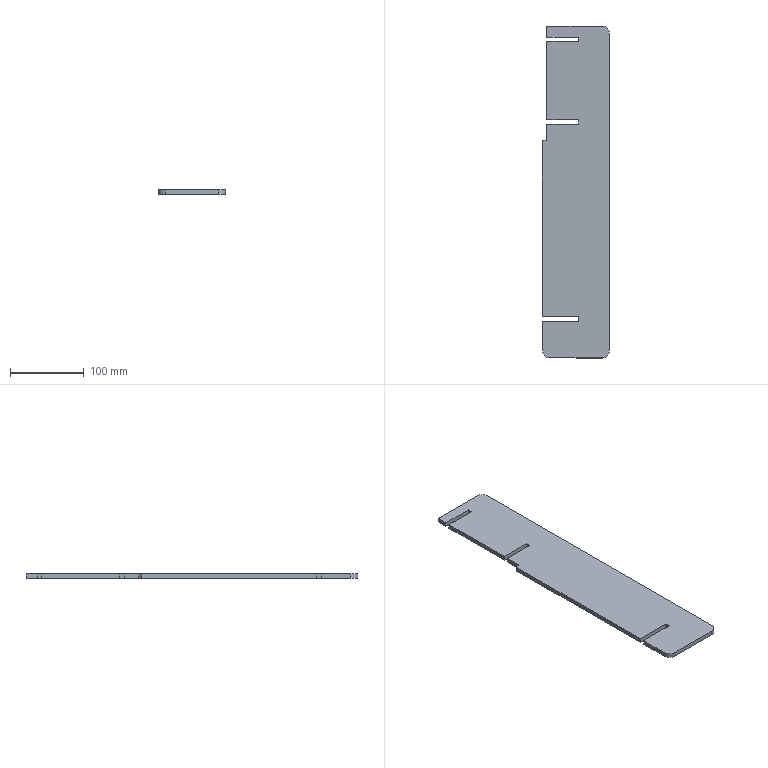Part | SolidWorks | features FlatPattern 1, SMBaseFlange 1, SheetMetal 1 | 1 solid | 25 faces | box 91 x 450 x 6 mm | volume 234874 mm3 | plane 20 | cylinder 5 | commonest cylinder face diameters 20 x3 4 x2
STEP:
#1=CARTESIAN_POINT('',(508.5,249.356,0.));
#2=VERTEX_POINT('',#1);
#3=CARTESIAN_POINT('',(508.5,234.356,0.));
#4=VERTEX_POINT('',#3);
#5=CARTESIAN_POINT('',(508.5,249.356,0.));
#6=DIRECTION('',(0.,-1.,0.));
#7=VECTOR('',#6,1000.);
#8=LINE('',#5,#7);
#9=EDGE_CURVE('',#2,#4,#8,.T.);
#10=ORIENTED_EDGE('',*,*,#9,.T.);
#11=CARTESIAN_POINT('',(508.5,234.356,6.));
#12=VERTEX_POINT('',#11);
#13=CARTESIAN_POINT('',(508.5,234.356,6.));
#14=DIRECTION('',(0.,0.,-1.));
#15=VECTOR('',#14,1000.);
#16=LINE('',#13,#15);
#17=EDGE_CURVE('',#12,#4,#16,.T.);
#18=ORIENTED_EDGE('',*,*,#17,.F.);
#19=CARTESIAN_POINT('',(508.5,249.356,6.));
#20=VERTEX_POINT('',#19);
#21=CARTESIAN_POINT('',(508.5,249.356,6.));
#22=DIRECTION('',(0.,-1.,0.));
#23=VECTOR('',#22,1000.);
#24=LINE('',#21,#23);
#25=EDGE_CURVE('',#20,#12,#24,.T.);
#26=ORIENTED_EDGE('',*,*,#25,.F.);
#27=CARTESIAN_POINT('',(508.5,249.356,6.));
#28=DIRECTION('',(0.,0.,-1.));
#29=VECTOR('',#28,1000.);
#30=LINE('',#27,#29);
#31=EDGE_CURVE('',#20,#2,#30,.T.);
#32=ORIENTED_EDGE('',*,*,#31,.T.);
#33=EDGE_LOOP('',(#10,#18,#26,#32));
#34=FACE_OUTER_BOUND('',#33,.T.);
#35=CARTESIAN_POINT('',(508.5,249.356,6.));
#36=DIRECTION('',(1.,0.,0.));
#37=DIRECTION('',(0.,0.,-1.));
#38=AXIS2_PLACEMENT_3D('',#35,#36,#37);
#39=PLANE('',#38);
#40=ADVANCED_FACE('',(#34),#39,.F.);
#41=CARTESIAN_POINT('',(551.5,234.356,0.));
#42=VERTEX_POINT('',#41);
#43=CARTESIAN_POINT('',(508.5,234.356,0.));
#44=DIRECTION('',(1.,0.,0.));
#45=VECTOR('',#44,1000.);
#46=LINE('',#43,#45);
#47=EDGE_CURVE('',#4,#42,#46,.T.);
#48=ORIENTED_EDGE('',*,*,#47,.T.);
#49=CARTESIAN_POINT('',(551.5,234.356,6.));
#50=VERTEX_POINT('',#49);
#51=CARTESIAN_POINT('',(551.5,234.356,6.));
#52=DIRECTION('',(0.,0.,-1.));
#53=VECTOR('',#52,1000.);
#54=LINE('',#51,#53);
#55=EDGE_CURVE('',#50,#42,#54,.T.);
#56=ORIENTED_EDGE('',*,*,#55,.F.);
#57=CARTESIAN_POINT('',(508.5,234.356,6.));
#58=DIRECTION('',(1.,0.,0.));
#59=VECTOR('',#58,1000.);
#60=LINE('',#57,#59);
#61=EDGE_CURVE('',#12,#50,#60,.T.);
#62=ORIENTED_EDGE('',*,*,#61,.F.);
#63=ORIENTED_EDGE('',*,*,#17,.T.);
#64=EDGE_LOOP('',(#48,#56,#62,#63));
#65=FACE_OUTER_BOUND('',#64,.T.);
#66=CARTESIAN_POINT('',(508.5,234.356,6.));
#67=DIRECTION('',(0.,1.,0.));
#68=DIRECTION('',(0.,0.,1.));
#69=AXIS2_PLACEMENT_3D('',#66,#67,#68);
#70=PLANE('',#69);
#71=ADVANCED_FACE('',(#65),#70,.F.);
#72=CARTESIAN_POINT('',(551.5,228.356,0.));
#73=VERTEX_POINT('',#72);
#74=CARTESIAN_POINT('',(551.5,234.356,0.));
#75=DIRECTION('',(0.,-1.,0.));
#76=VECTOR('',#75,1000.);
#77=LINE('',#74,#76);
#78=EDGE_CURVE('',#42,#73,#77,.T.);
#79=ORIENTED_EDGE('',*,*,#78,.T.);
#80=CARTESIAN_POINT('',(551.5,228.356,6.));
#81=VERTEX_POINT('',#80);
#82=CARTESIAN_POINT('',(551.5,228.356,6.));
#83=DIRECTION('',(0.,0.,-1.));
#84=VECTOR('',#83,1000.);
#85=LINE('',#82,#84);
#86=EDGE_CURVE('',#81,#73,#85,.T.);
#87=ORIENTED_EDGE('',*,*,#86,.F.);
#88=CARTESIAN_POINT('',(551.5,234.356,6.));
#89=DIRECTION('',(0.,-1.,0.));
#90=VECTOR('',#89,1000.);
#91=LINE('',#88,#90);
#92=EDGE_CURVE('',#50,#81,#91,.T.);
#93=ORIENTED_EDGE('',*,*,#92,.F.);
#94=ORIENTED_EDGE('',*,*,#55,.T.);
#95=EDGE_LOOP('',(#79,#87,#93,#94));
#96=FACE_OUTER_BOUND('',#95,.T.);
#97=CARTESIAN_POINT('',(551.5,234.356,6.));
#98=DIRECTION('',(1.,0.,0.));
#99=DIRECTION('',(0.,0.,-1.));
#100=AXIS2_PLACEMENT_3D('',#97,#98,#99);
#101=PLANE('',#100);
#102=ADVANCED_FACE('',(#96),#101,.F.);
#103=CARTESIAN_POINT('',(508.5,228.356,0.));
#104=VERTEX_POINT('',#103);
#105=CARTESIAN_POINT('',(551.5,228.356,0.));
#106=DIRECTION('',(-1.,0.,0.));
#107=VECTOR('',#106,1000.);
#108=LINE('',#105,#107);
#109=EDGE_CURVE('',#73,#104,#108,.T.);
#110=ORIENTED_EDGE('',*,*,#109,.T.);
#111=CARTESIAN_POINT('',(508.5,228.356,6.));
#112=VERTEX_POINT('',#111);
#113=CARTESIAN_POINT('',(508.5,228.356,6.));
#114=DIRECTION('',(0.,0.,-1.));
#115=VECTOR('',#114,1000.);
#116=LINE('',#113,#115);
#117=EDGE_CURVE('',#112,#104,#116,.T.);
#118=ORIENTED_EDGE('',*,*,#117,.F.);
#119=CARTESIAN_POINT('',(551.5,228.356,6.));
#120=DIRECTION('',(-1.,0.,0.));
#121=VECTOR('',#120,1000.);
#122=LINE('',#119,#121);
#123=EDGE_CURVE('',#81,#112,#122,.T.);
#124=ORIENTED_EDGE('',*,*,#123,.F.);
#125=ORIENTED_EDGE('',*,*,#86,.T.);
#126=EDGE_LOOP('',(#110,#118,#124,#125));
#127=FACE_OUTER_BOUND('',#126,.T.);
#128=CARTESIAN_POINT('',(551.5,228.356,6.));
#129=DIRECTION('',(0.,-1.,0.));
#130=DIRECTION('',(0.,0.,-1.));
#131=AXIS2_PLACEMENT_3D('',#128,#129,#130);
#132=PLANE('',#131);
#133=ADVANCED_FACE('',(#127),#132,.F.);
#134=CARTESIAN_POINT('',(508.5,122.356,0.));
#135=VERTEX_POINT('',#134);
#136=CARTESIAN_POINT('',(508.5,228.356,0.));
#137=DIRECTION('',(0.,-1.,0.));
#138=VECTOR('',#137,1000.);
#139=LINE('',#136,#138);
#140=EDGE_CURVE('',#104,#135,#139,.T.);
#141=ORIENTED_EDGE('',*,*,#140,.T.);
#142=CARTESIAN_POINT('',(508.5,122.356,6.));
#143=VERTEX_POINT('',#142);
#144=CARTESIAN_POINT('',(508.5,122.356,6.));
#145=DIRECTION('',(0.,0.,-1.));
#146=VECTOR('',#145,1000.);
#147=LINE('',#144,#146);
#148=EDGE_CURVE('',#143,#135,#147,.T.);
#149=ORIENTED_EDGE('',*,*,#148,.F.);
#150=CARTESIAN_POINT('',(508.5,228.356,6.));
#151=DIRECTION('',(0.,-1.,0.));
#152=VECTOR('',#151,1000.);
#153=LINE('',#150,#152);
#154=EDGE_CURVE('',#112,#143,#153,.T.);
#155=ORIENTED_EDGE('',*,*,#154,.F.);
#156=ORIENTED_EDGE('',*,*,#117,.T.);
#157=EDGE_LOOP('',(#141,#149,#155,#156));
#158=FACE_OUTER_BOUND('',#157,.T.);
#159=CARTESIAN_POINT('',(508.5,228.356,6.));
#160=DIRECTION('',(1.,0.,0.));
#161=DIRECTION('',(0.,0.,-1.));
#162=AXIS2_PLACEMENT_3D('',#159,#160,#161);
#163=PLANE('',#162);
#164=ADVANCED_FACE('',(#158),#163,.F.);
#165=CARTESIAN_POINT('',(551.5,122.356,0.));
#166=VERTEX_POINT('',#165);
#167=CARTESIAN_POINT('',(508.5,122.356,0.));
#168=DIRECTION('',(1.,0.,0.));
#169=VECTOR('',#168,1000.);
#170=LINE('',#167,#169);
#171=EDGE_CURVE('',#135,#166,#170,.T.);
#172=ORIENTED_EDGE('',*,*,#171,.T.);
#173=CARTESIAN_POINT('',(551.5,122.356,6.));
#174=VERTEX_POINT('',#173);
#175=CARTESIAN_POINT('',(551.5,122.356,6.));
#176=DIRECTION('',(0.,0.,-1.));
#177=VECTOR('',#176,1000.);
#178=LINE('',#175,#177);
#179=EDGE_CURVE('',#174,#166,#178,.T.);
#180=ORIENTED_EDGE('',*,*,#179,.F.);
#181=CARTESIAN_POINT('',(508.5,122.356,6.));
#182=DIRECTION('',(1.,0.,0.));
#183=VECTOR('',#182,1000.);
#184=LINE('',#181,#183);
#185=EDGE_CURVE('',#143,#174,#184,.T.);
#186=ORIENTED_EDGE('',*,*,#185,.F.);
#187=ORIENTED_EDGE('',*,*,#148,.T.);
#188=EDGE_LOOP('',(#172,#180,#186,#187));
#189=FACE_OUTER_BOUND('',#188,.T.);
#190=CARTESIAN_POINT('',(508.5,122.356,6.));
#191=DIRECTION('',(0.,1.,0.));
#192=DIRECTION('',(0.,0.,1.));
#193=AXIS2_PLACEMENT_3D('',#190,#191,#192);
#194=PLANE('',#193);
#195=ADVANCED_FACE('',(#189),#194,.F.);
#196=CARTESIAN_POINT('',(551.5,116.356,0.));
#197=VERTEX_POINT('',#196);
#198=CARTESIAN_POINT('',(551.5,122.356,0.));
#199=DIRECTION('',(0.,-1.,0.));
#200=VECTOR('',#199,1000.);
#201=LINE('',#198,#200);
#202=EDGE_CURVE('',#166,#197,#201,.T.);
#203=ORIENTED_EDGE('',*,*,#202,.T.);
#204=CARTESIAN_POINT('',(551.5,116.356,6.));
#205=VERTEX_POINT('',#204);
#206=CARTESIAN_POINT('',(551.5,116.356,6.));
#207=DIRECTION('',(0.,0.,-1.));
#208=VECTOR('',#207,1000.);
#209=LINE('',#206,#208);
#210=EDGE_CURVE('',#205,#197,#209,.T.);
#211=ORIENTED_EDGE('',*,*,#210,.F.);
#212=CARTESIAN_POINT('',(551.5,122.356,6.));
#213=DIRECTION('',(0.,-1.,0.));
#214=VECTOR('',#213,1000.);
#215=LINE('',#212,#214);
#216=EDGE_CURVE('',#174,#205,#215,.T.);
#217=ORIENTED_EDGE('',*,*,#216,.F.);
#218=ORIENTED_EDGE('',*,*,#179,.T.);
#219=EDGE_LOOP('',(#203,#211,#217,#218));
#220=FACE_OUTER_BOUND('',#219,.T.);
#221=CARTESIAN_POINT('',(551.5,122.356,6.));
#222=DIRECTION('',(1.,0.,0.));
#223=DIRECTION('',(0.,0.,-1.));
#224=AXIS2_PLACEMENT_3D('',#221,#222,#223);
#225=PLANE('',#224);
#226=ADVANCED_FACE('',(#220),#225,.F.);
#227=CARTESIAN_POINT('',(508.5,116.356,0.));
#228=VERTEX_POINT('',#227);
#229=CARTESIAN_POINT('',(551.5,116.356,0.));
#230=DIRECTION('',(-1.,0.,0.));
#231=VECTOR('',#230,1000.);
#232=LINE('',#229,#231);
#233=EDGE_CURVE('',#197,#228,#232,.T.);
#234=ORIENTED_EDGE('',*,*,#233,.T.);
#235=CARTESIAN_POINT('',(508.5,116.356,6.));
#236=VERTEX_POINT('',#235);
#237=CARTESIAN_POINT('',(508.5,116.356,6.));
#238=DIRECTION('',(0.,0.,-1.));
#239=VECTOR('',#238,1000.);
#240=LINE('',#237,#239);
#241=EDGE_CURVE('',#236,#228,#240,.T.);
#242=ORIENTED_EDGE('',*,*,#241,.F.);
#243=CARTESIAN_POINT('',(551.5,116.356,6.));
#244=DIRECTION('',(-1.,0.,0.));
#245=VECTOR('',#244,1000.);
#246=LINE('',#243,#245);
#247=EDGE_CURVE('',#205,#236,#246,.T.);
#248=ORIENTED_EDGE('',*,*,#247,.F.);
#249=ORIENTED_EDGE('',*,*,#210,.T.);
#250=EDGE_LOOP('',(#234,#242,#248,#249));
#251=FACE_OUTER_BOUND('',#250,.T.);
#252=CARTESIAN_POINT('',(551.5,116.356,6.));
#253=DIRECTION('',(0.,-1.,0.));
#254=DIRECTION('',(0.,0.,-1.));
#255=AXIS2_PLACEMENT_3D('',#252,#253,#254);
#256=PLANE('',#255);
#257=ADVANCED_FACE('',(#251),#256,.F.);
#258=CARTESIAN_POINT('',(508.5,96.356,0.));
#259=VERTEX_POINT('',#258);
#260=CARTESIAN_POINT('',(508.5,116.356,0.));
#261=DIRECTION('',(0.,-1.,0.));
#262=VECTOR('',#261,1000.);
#263=LINE('',#260,#262);
#264=EDGE_CURVE('',#228,#259,#263,.T.);
#265=ORIENTED_EDGE('',*,*,#264,.T.);
#266=CARTESIAN_POINT('',(508.5,96.356,6.));
#267=VERTEX_POINT('',#266);
#268=CARTESIAN_POINT('',(508.5,96.356,6.));
#269=DIRECTION('',(0.,0.,-1.));
#270=VECTOR('',#269,1000.);
#271=LINE('',#268,#270);
#272=EDGE_CURVE('',#267,#259,#271,.T.);
#273=ORIENTED_EDGE('',*,*,#272,.F.);
#274=CARTESIAN_POINT('',(508.5,116.356,6.));
#275=DIRECTION('',(0.,-1.,0.));
#276=VECTOR('',#275,1000.);
#277=LINE('',#274,#276);
#278=EDGE_CURVE('',#236,#267,#277,.T.);
#279=ORIENTED_EDGE('',*,*,#278,.F.);
#280=ORIENTED_EDGE('',*,*,#241,.T.);
#281=EDGE_LOOP('',(#265,#273,#279,#280));
#282=FACE_OUTER_BOUND('',#281,.T.);
#283=CARTESIAN_POINT('',(508.5,116.356,6.));
#284=DIRECTION('',(1.,0.,0.));
#285=DIRECTION('',(0.,0.,-1.));
#286=AXIS2_PLACEMENT_3D('',#283,#284,#285);
#287=PLANE('',#286);
#288=ADVANCED_FACE('',(#282),#287,.F.);
#289=CARTESIAN_POINT('',(506.5,94.356,0.));
#290=VERTEX_POINT('',#289);
#291=CARTESIAN_POINT('',(506.5,96.356,0.));
#292=DIRECTION('',(0.,0.,-1.));
#293=DIRECTION('',(-1.,0.,0.));
#294=AXIS2_PLACEMENT_3D('',#291,#292,#293);
#295=CIRCLE('',#294,2.);
#296=EDGE_CURVE('',#259,#290,#295,.T.);
#297=ORIENTED_EDGE('',*,*,#296,.T.);
#298=CARTESIAN_POINT('',(506.5,94.356,6.));
#299=VERTEX_POINT('',#298);
#300=CARTESIAN_POINT('',(506.5,94.356,6.));
#301=DIRECTION('',(0.,0.,-1.));
#302=VECTOR('',#301,1000.);
#303=LINE('',#300,#302);
#304=EDGE_CURVE('',#299,#290,#303,.T.);
#305=ORIENTED_EDGE('',*,*,#304,.F.);
#306=CARTESIAN_POINT('',(506.5,96.356,6.));
#307=DIRECTION('',(0.,0.,-1.));
#308=DIRECTION('',(-1.,0.,0.));
#309=AXIS2_PLACEMENT_3D('',#306,#307,#308);
#310=CIRCLE('',#309,2.);
#311=EDGE_CURVE('',#267,#299,#310,.T.);
#312=ORIENTED_EDGE('',*,*,#311,.F.);
#313=ORIENTED_EDGE('',*,*,#272,.T.);
#314=EDGE_LOOP('',(#297,#305,#312,#313));
#315=FACE_OUTER_BOUND('',#314,.T.);
#316=CARTESIAN_POINT('',(506.5,96.356,6.));
#317=DIRECTION('',(0.,0.,-1.));
#318=DIRECTION('',(-1.,0.,0.));
#319=AXIS2_PLACEMENT_3D('',#316,#317,#318);
#320=CYLINDRICAL_SURFACE('',#319,2.);
#321=ADVANCED_FACE('',(#315),#320,.F.);
#322=CARTESIAN_POINT('',(504.5,94.356,0.));
#323=VERTEX_POINT('',#322);
#324=CARTESIAN_POINT('',(506.5,94.356,0.));
#325=DIRECTION('',(-1.,0.,0.));
#326=VECTOR('',#325,1000.);
#327=LINE('',#324,#326);
#328=EDGE_CURVE('',#290,#323,#327,.T.);
#329=ORIENTED_EDGE('',*,*,#328,.T.);
#330=CARTESIAN_POINT('',(504.5,94.356,6.));
#331=VERTEX_POINT('',#330);
#332=CARTESIAN_POINT('',(504.5,94.356,6.));
#333=DIRECTION('',(0.,0.,-1.));
#334=VECTOR('',#333,1000.);
#335=LINE('',#332,#334);
#336=EDGE_CURVE('',#331,#323,#335,.T.);
#337=ORIENTED_EDGE('',*,*,#336,.F.);
#338=CARTESIAN_POINT('',(506.5,94.356,6.));
#339=DIRECTION('',(-1.,0.,0.));
#340=VECTOR('',#339,1000.);
#341=LINE('',#338,#340);
#342=EDGE_CURVE('',#299,#331,#341,.T.);
#343=ORIENTED_EDGE('',*,*,#342,.F.);
#344=ORIENTED_EDGE('',*,*,#304,.T.);
#345=EDGE_LOOP('',(#329,#337,#343,#344));
#346=FACE_OUTER_BOUND('',#345,.T.);
#347=CARTESIAN_POINT('',(506.5,94.356,6.));
#348=DIRECTION('',(0.,-1.,0.));
#349=DIRECTION('',(1.,0.,0.));
#350=AXIS2_PLACEMENT_3D('',#347,#348,#349);
#351=PLANE('',#350);
#352=ADVANCED_FACE('',(#346),#351,.F.);
#353=CARTESIAN_POINT('',(502.5,92.356,0.));
#354=VERTEX_POINT('',#353);
#355=CARTESIAN_POINT('',(504.5,92.356,0.));
#356=DIRECTION('',(0.,0.,1.));
#357=DIRECTION('',(1.,0.,0.));
#358=AXIS2_PLACEMENT_3D('',#355,#356,#357);
#359=CIRCLE('',#358,2.);
#360=EDGE_CURVE('',#323,#354,#359,.T.);
#361=ORIENTED_EDGE('',*,*,#360,.T.);
#362=CARTESIAN_POINT('',(502.5,92.356,6.));
#363=VERTEX_POINT('',#362);
#364=CARTESIAN_POINT('',(502.5,92.356,6.));
#365=DIRECTION('',(0.,0.,-1.));
#366=VECTOR('',#365,1000.);
#367=LINE('',#364,#366);
#368=EDGE_CURVE('',#363,#354,#367,.T.);
#369=ORIENTED_EDGE('',*,*,#368,.F.);
#370=CARTESIAN_POINT('',(504.5,92.356,6.));
#371=DIRECTION('',(0.,0.,1.));
#372=DIRECTION('',(1.,0.,0.));
#373=AXIS2_PLACEMENT_3D('',#370,#371,#372);
#374=CIRCLE('',#373,2.);
#375=EDGE_CURVE('',#331,#363,#374,.T.);
#376=ORIENTED_EDGE('',*,*,#375,.F.);
#377=ORIENTED_EDGE('',*,*,#336,.T.);
#378=EDGE_LOOP('',(#361,#369,#376,#377));
#379=FACE_OUTER_BOUND('',#378,.T.);
#380=CARTESIAN_POINT('',(504.5,92.356,6.));
#381=DIRECTION('',(0.,0.,-1.));
#382=DIRECTION('',(-1.,0.,0.));
#383=AXIS2_PLACEMENT_3D('',#380,#381,#382);
#384=CYLINDRICAL_SURFACE('',#383,2.);
#385=ADVANCED_FACE('',(#379),#384,.T.);
#386=CARTESIAN_POINT('',(502.5,-144.644,0.));
#387=VERTEX_POINT('',#386);
#388=CARTESIAN_POINT('',(502.5,92.356,0.));
#389=DIRECTION('',(0.,-1.,0.));
#390=VECTOR('',#389,1000.);
#391=LINE('',#388,#390);
#392=EDGE_CURVE('',#354,#387,#391,.T.);
#393=ORIENTED_EDGE('',*,*,#392,.T.);
#394=CARTESIAN_POINT('',(502.5,-144.644,6.));
#395=VERTEX_POINT('',#394);
#396=CARTESIAN_POINT('',(502.5,-144.644,6.));
#397=DIRECTION('',(0.,0.,-1.));
#398=VECTOR('',#397,1000.);
#399=LINE('',#396,#398);
#400=EDGE_CURVE('',#395,#387,#399,.T.);
#401=ORIENTED_EDGE('',*,*,#400,.F.);
#402=CARTESIAN_POINT('',(502.5,92.356,6.));
#403=DIRECTION('',(0.,-1.,0.));
#404=VECTOR('',#403,1000.);
#405=LINE('',#402,#404);
#406=EDGE_CURVE('',#363,#395,#405,.T.);
#407=ORIENTED_EDGE('',*,*,#406,.F.);
#408=ORIENTED_EDGE('',*,*,#368,.T.);
#409=EDGE_LOOP('',(#393,#401,#407,#408));
#410=FACE_OUTER_BOUND('',#409,.T.);
#411=CARTESIAN_POINT('',(502.5,92.356,6.));
#412=DIRECTION('',(1.,0.,0.));
#413=DIRECTION('',(0.,0.,-1.));
#414=AXIS2_PLACEMENT_3D('',#411,#412,#413);
#415=PLANE('',#414);
#416=ADVANCED_FACE('',(#410),#415,.F.);
#417=CARTESIAN_POINT('',(551.5,-144.644,0.));
#418=VERTEX_POINT('',#417);
#419=CARTESIAN_POINT('',(502.5,-144.644,0.));
#420=DIRECTION('',(1.,0.,0.));
#421=VECTOR('',#420,1000.);
#422=LINE('',#419,#421);
#423=EDGE_CURVE('',#387,#418,#422,.T.);
#424=ORIENTED_EDGE('',*,*,#423,.T.);
#425=CARTESIAN_POINT('',(551.5,-144.644,6.));
#426=VERTEX_POINT('',#425);
#427=CARTESIAN_POINT('',(551.5,-144.644,6.));
#428=DIRECTION('',(0.,0.,-1.));
#429=VECTOR('',#428,1000.);
#430=LINE('',#427,#429);
#431=EDGE_CURVE('',#426,#418,#430,.T.);
#432=ORIENTED_EDGE('',*,*,#431,.F.);
#433=CARTESIAN_POINT('',(502.5,-144.644,6.));
#434=DIRECTION('',(1.,0.,0.));
#435=VECTOR('',#434,1000.);
#436=LINE('',#433,#435);
#437=EDGE_CURVE('',#395,#426,#436,.T.);
#438=ORIENTED_EDGE('',*,*,#437,.F.);
#439=ORIENTED_EDGE('',*,*,#400,.T.);
#440=EDGE_LOOP('',(#424,#432,#438,#439));
#441=FACE_OUTER_BOUND('',#440,.T.);
#442=CARTESIAN_POINT('',(502.5,-144.644,6.));
#443=DIRECTION('',(0.,1.,0.));
#444=DIRECTION('',(0.,0.,1.));
#445=AXIS2_PLACEMENT_3D('',#442,#443,#444);
#446=PLANE('',#445);
#447=ADVANCED_FACE('',(#441),#446,.F.);
#448=CARTESIAN_POINT('',(551.5,-150.644,0.));
#449=VERTEX_POINT('',#448);
#450=CARTESIAN_POINT('',(551.5,-144.644,0.));
#451=DIRECTION('',(0.,-1.,0.));
#452=VECTOR('',#451,1000.);
#453=LINE('',#450,#452);
#454=EDGE_CURVE('',#418,#449,#453,.T.);
#455=ORIENTED_EDGE('',*,*,#454,.T.);
#456=CARTESIAN_POINT('',(551.5,-150.644,6.));
#457=VERTEX_POINT('',#456);
#458=CARTESIAN_POINT('',(551.5,-150.644,6.));
#459=DIRECTION('',(0.,0.,-1.));
#460=VECTOR('',#459,1000.);
#461=LINE('',#458,#460);
#462=EDGE_CURVE('',#457,#449,#461,.T.);
#463=ORIENTED_EDGE('',*,*,#462,.F.);
#464=CARTESIAN_POINT('',(551.5,-144.644,6.));
#465=DIRECTION('',(0.,-1.,0.));
#466=VECTOR('',#465,1000.);
#467=LINE('',#464,#466);
#468=EDGE_CURVE('',#426,#457,#467,.T.);
#469=ORIENTED_EDGE('',*,*,#468,.F.);
#470=ORIENTED_EDGE('',*,*,#431,.T.);
#471=EDGE_LOOP('',(#455,#463,#469,#470));
#472=FACE_OUTER_BOUND('',#471,.T.);
#473=CARTESIAN_POINT('',(551.5,-144.644,6.));
#474=DIRECTION('',(1.,0.,0.));
#475=DIRECTION('',(0.,0.,-1.));
#476=AXIS2_PLACEMENT_3D('',#473,#474,#475);
#477=PLANE('',#476);
#478=ADVANCED_FACE('',(#472),#477,.F.);
#479=CARTESIAN_POINT('',(502.5,-150.644,0.));
#480=VERTEX_POINT('',#479);
#481=CARTESIAN_POINT('',(551.5,-150.644,0.));
#482=DIRECTION('',(-1.,0.,0.));
#483=VECTOR('',#482,1000.);
#484=LINE('',#481,#483);
#485=EDGE_CURVE('',#449,#480,#484,.T.);
#486=ORIENTED_EDGE('',*,*,#485,.T.);
#487=CARTESIAN_POINT('',(502.5,-150.644,6.));
#488=VERTEX_POINT('',#487);
#489=CARTESIAN_POINT('',(502.5,-150.644,6.));
#490=DIRECTION('',(0.,0.,-1.));
#491=VECTOR('',#490,1000.);
#492=LINE('',#489,#491);
#493=EDGE_CURVE('',#488,#480,#492,.T.);
#494=ORIENTED_EDGE('',*,*,#493,.F.);
#495=CARTESIAN_POINT('',(551.5,-150.644,6.));
#496=DIRECTION('',(-1.,0.,0.));
#497=VECTOR('',#496,1000.);
#498=LINE('',#495,#497);
#499=EDGE_CURVE('',#457,#488,#498,.T.);
#500=ORIENTED_EDGE('',*,*,#499,.F.);
#501=ORIENTED_EDGE('',*,*,#462,.T.);
#502=EDGE_LOOP('',(#486,#494,#500,#501));
#503=FACE_OUTER_BOUND('',#502,.T.);
#504=CARTESIAN_POINT('',(551.5,-150.644,6.));
#505=DIRECTION('',(0.,-1.,0.));
#506=DIRECTION('',(0.,0.,-1.));
#507=AXIS2_PLACEMENT_3D('',#504,#505,#506);
#508=PLANE('',#507);
#509=ADVANCED_FACE('',(#503),#508,.F.);
#510=CARTESIAN_POINT('',(502.5,-190.644,0.));
#511=VERTEX_POINT('',#510);
#512=CARTESIAN_POINT('',(502.5,-150.644,0.));
#513=DIRECTION('',(0.,-1.,0.));
#514=VECTOR('',#513,1000.);
#515=LINE('',#512,#514);
#516=EDGE_CURVE('',#480,#511,#515,.T.);
#517=ORIENTED_EDGE('',*,*,#516,.T.);
#518=CARTESIAN_POINT('',(502.5,-190.644,6.));
#519=VERTEX_POINT('',#518);
#520=CARTESIAN_POINT('',(502.5,-190.644,6.));
#521=DIRECTION('',(0.,0.,-1.));
#522=VECTOR('',#521,1000.);
#523=LINE('',#520,#522);
#524=EDGE_CURVE('',#519,#511,#523,.T.);
#525=ORIENTED_EDGE('',*,*,#524,.F.);
#526=CARTESIAN_POINT('',(502.5,-150.644,6.));
#527=DIRECTION('',(0.,-1.,0.));
#528=VECTOR('',#527,1000.);
#529=LINE('',#526,#528);
#530=EDGE_CURVE('',#488,#519,#529,.T.);
#531=ORIENTED_EDGE('',*,*,#530,.F.);
#532=ORIENTED_EDGE('',*,*,#493,.T.);
#533=EDGE_LOOP('',(#517,#525,#531,#532));
#534=FACE_OUTER_BOUND('',#533,.T.);
#535=CARTESIAN_POINT('',(502.5,-150.644,6.));
#536=DIRECTION('',(1.,0.,0.));
#537=DIRECTION('',(0.,1.,0.));
#538=AXIS2_PLACEMENT_3D('',#535,#536,#537);
#539=PLANE('',#538);
#540=ADVANCED_FACE('',(#534),#539,.F.);
#541=CARTESIAN_POINT('',(512.5,-200.644,0.));
#542=VERTEX_POINT('',#541);
#543=CARTESIAN_POINT('',(512.5,-190.644,0.));
#544=DIRECTION('',(0.,0.,1.));
#545=DIRECTION('',(1.,0.,0.));
#546=AXIS2_PLACEMENT_3D('',#543,#544,#545);
#547=CIRCLE('',#546,10.);
#548=EDGE_CURVE('',#511,#542,#547,.T.);
#549=ORIENTED_EDGE('',*,*,#548,.T.);
#550=CARTESIAN_POINT('',(512.5,-200.644,6.));
#551=VERTEX_POINT('',#550);
#552=CARTESIAN_POINT('',(512.5,-200.644,6.));
#553=DIRECTION('',(0.,0.,-1.));
#554=VECTOR('',#553,1000.);
#555=LINE('',#552,#554);
#556=EDGE_CURVE('',#551,#542,#555,.T.);
#557=ORIENTED_EDGE('',*,*,#556,.F.);
#558=CARTESIAN_POINT('',(512.5,-190.644,6.));
#559=DIRECTION('',(0.,0.,1.));
#560=DIRECTION('',(1.,0.,0.));
#561=AXIS2_PLACEMENT_3D('',#558,#559,#560);
#562=CIRCLE('',#561,10.);
#563=EDGE_CURVE('',#519,#551,#562,.T.);
#564=ORIENTED_EDGE('',*,*,#563,.F.);
#565=ORIENTED_EDGE('',*,*,#524,.T.);
#566=EDGE_LOOP('',(#549,#557,#564,#565));
#567=FACE_OUTER_BOUND('',#566,.T.);
#568=CARTESIAN_POINT('',(512.5,-190.644,6.));
#569=DIRECTION('',(0.,0.,-1.));
#570=DIRECTION('',(-1.,0.,0.));
#571=AXIS2_PLACEMENT_3D('',#568,#569,#570);
#572=CYLINDRICAL_SURFACE('',#571,10.);
#573=ADVANCED_FACE('',(#567),#572,.T.);
#574=CARTESIAN_POINT('',(583.5,-200.644,0.));
#575=VERTEX_POINT('',#574);
#576=CARTESIAN_POINT('',(512.5,-200.644,0.));
#577=DIRECTION('',(1.,0.,0.));
#578=VECTOR('',#577,1000.);
#579=LINE('',#576,#578);
#580=EDGE_CURVE('',#542,#575,#579,.T.);
#581=ORIENTED_EDGE('',*,*,#580,.T.);
#582=CARTESIAN_POINT('',(583.5,-200.644,6.));
#583=VERTEX_POINT('',#582);
#584=CARTESIAN_POINT('',(583.5,-200.644,6.));
#585=DIRECTION('',(0.,0.,-1.));
#586=VECTOR('',#585,1000.);
#587=LINE('',#584,#586);
#588=EDGE_CURVE('',#583,#575,#587,.T.);
#589=ORIENTED_EDGE('',*,*,#588,.F.);
#590=CARTESIAN_POINT('',(512.5,-200.644,6.));
#591=DIRECTION('',(1.,0.,0.));
#592=VECTOR('',#591,1000.);
#593=LINE('',#590,#592);
#594=EDGE_CURVE('',#551,#583,#593,.T.);
#595=ORIENTED_EDGE('',*,*,#594,.F.);
#596=ORIENTED_EDGE('',*,*,#556,.T.);
#597=EDGE_LOOP('',(#581,#589,#595,#596));
#598=FACE_OUTER_BOUND('',#597,.T.);
#599=CARTESIAN_POINT('',(512.5,-200.644,6.));
#600=DIRECTION('',(0.,1.,0.));
#601=DIRECTION('',(-1.,0.,0.));
#602=AXIS2_PLACEMENT_3D('',#599,#600,#601);
#603=PLANE('',#602);
#604=ADVANCED_FACE('',(#598),#603,.F.);
#605=CARTESIAN_POINT('',(593.5,-190.644,0.));
#606=VERTEX_POINT('',#605);
#607=CARTESIAN_POINT('',(583.5,-190.644,0.));
#608=DIRECTION('',(0.,0.,1.));
#609=DIRECTION('',(1.,0.,0.));
#610=AXIS2_PLACEMENT_3D('',#607,#608,#609);
#611=CIRCLE('',#610,10.);
#612=EDGE_CURVE('',#575,#606,#611,.T.);
#613=ORIENTED_EDGE('',*,*,#612,.T.);
#614=CARTESIAN_POINT('',(593.5,-190.644,6.));
#615=VERTEX_POINT('',#614);
#616=CARTESIAN_POINT('',(593.5,-190.644,6.));
#617=DIRECTION('',(0.,0.,-1.));
#618=VECTOR('',#617,1000.);
#619=LINE('',#616,#618);
#620=EDGE_CURVE('',#615,#606,#619,.T.);
#621=ORIENTED_EDGE('',*,*,#620,.F.);
#622=CARTESIAN_POINT('',(583.5,-190.644,6.));
#623=DIRECTION('',(0.,0.,1.));
#624=DIRECTION('',(1.,0.,0.));
#625=AXIS2_PLACEMENT_3D('',#622,#623,#624);
#626=CIRCLE('',#625,10.);
#627=EDGE_CURVE('',#583,#615,#626,.T.);
#628=ORIENTED_EDGE('',*,*,#627,.F.);
#629=ORIENTED_EDGE('',*,*,#588,.T.);
#630=EDGE_LOOP('',(#613,#621,#628,#629));
#631=FACE_OUTER_BOUND('',#630,.T.);
#632=CARTESIAN_POINT('',(583.5,-190.644,6.));
#633=DIRECTION('',(0.,0.,-1.));
#634=DIRECTION('',(-1.,0.,0.));
#635=AXIS2_PLACEMENT_3D('',#632,#633,#634);
#636=CYLINDRICAL_SURFACE('',#635,10.);
#637=ADVANCED_FACE('',(#631),#636,.T.);
#638=CARTESIAN_POINT('',(593.5,239.356,0.));
#639=VERTEX_POINT('',#638);
#640=CARTESIAN_POINT('',(593.5,-190.644,0.));
#641=DIRECTION('',(0.,1.,0.));
#642=VECTOR('',#641,1000.);
#643=LINE('',#640,#642);
#644=EDGE_CURVE('',#606,#639,#643,.T.);
#645=ORIENTED_EDGE('',*,*,#644,.T.);
#646=CARTESIAN_POINT('',(593.5,239.356,6.));
#647=VERTEX_POINT('',#646);
#648=CARTESIAN_POINT('',(593.5,239.356,6.));
#649=DIRECTION('',(0.,0.,-1.));
#650=VECTOR('',#649,1000.);
#651=LINE('',#648,#650);
#652=EDGE_CURVE('',#647,#639,#651,.T.);
#653=ORIENTED_EDGE('',*,*,#652,.F.);
#654=CARTESIAN_POINT('',(593.5,-190.644,6.));
#655=DIRECTION('',(0.,1.,0.));
#656=VECTOR('',#655,1000.);
#657=LINE('',#654,#656);
#658=EDGE_CURVE('',#615,#647,#657,.T.);
#659=ORIENTED_EDGE('',*,*,#658,.F.);
#660=ORIENTED_EDGE('',*,*,#620,.T.);
#661=EDGE_LOOP('',(#645,#653,#659,#660));
#662=FACE_OUTER_BOUND('',#661,.T.);
#663=CARTESIAN_POINT('',(593.5,-190.644,6.));
#664=DIRECTION('',(-1.,0.,0.));
#665=DIRECTION('',(0.,0.,1.));
#666=AXIS2_PLACEMENT_3D('',#663,#664,#665);
#667=PLANE('',#666);
#668=ADVANCED_FACE('',(#662),#667,.F.);
#669=CARTESIAN_POINT('',(583.5,249.356,0.));
#670=VERTEX_POINT('',#669);
#671=CARTESIAN_POINT('',(583.5,239.356,0.));
#672=DIRECTION('',(0.,0.,1.));
#673=DIRECTION('',(-1.,0.,0.));
#674=AXIS2_PLACEMENT_3D('',#671,#672,#673);
#675=CIRCLE('',#674,10.);
#676=EDGE_CURVE('',#639,#670,#675,.T.);
#677=ORIENTED_EDGE('',*,*,#676,.T.);
#678=CARTESIAN_POINT('',(583.5,249.356,6.));
#679=VERTEX_POINT('',#678);
#680=CARTESIAN_POINT('',(583.5,249.356,6.));
#681=DIRECTION('',(0.,0.,-1.));
#682=VECTOR('',#681,1000.);
#683=LINE('',#680,#682);
#684=EDGE_CURVE('',#679,#670,#683,.T.);
#685=ORIENTED_EDGE('',*,*,#684,.F.);
#686=CARTESIAN_POINT('',(583.5,239.356,6.));
#687=DIRECTION('',(0.,0.,1.));
#688=DIRECTION('',(-1.,0.,0.));
#689=AXIS2_PLACEMENT_3D('',#686,#687,#688);
#690=CIRCLE('',#689,10.);
#691=EDGE_CURVE('',#647,#679,#690,.T.);
#692=ORIENTED_EDGE('',*,*,#691,.F.);
#693=ORIENTED_EDGE('',*,*,#652,.T.);
#694=EDGE_LOOP('',(#677,#685,#692,#693));
#695=FACE_OUTER_BOUND('',#694,.T.);
#696=CARTESIAN_POINT('',(583.5,239.356,6.));
#697=DIRECTION('',(0.,0.,-1.));
#698=DIRECTION('',(-1.,0.,0.));
#699=AXIS2_PLACEMENT_3D('',#696,#697,#698);
#700=CYLINDRICAL_SURFACE('',#699,10.);
#701=ADVANCED_FACE('',(#695),#700,.T.);
#702=CARTESIAN_POINT('',(583.5,249.356,0.));
#703=DIRECTION('',(-1.,0.,0.));
#704=VECTOR('',#703,1000.);
#705=LINE('',#702,#704);
#706=EDGE_CURVE('',#670,#2,#705,.T.);
#707=ORIENTED_EDGE('',*,*,#706,.T.);
#708=ORIENTED_EDGE('',*,*,#31,.F.);
#709=CARTESIAN_POINT('',(583.5,249.356,6.));
#710=DIRECTION('',(-1.,0.,0.));
#711=VECTOR('',#710,1000.);
#712=LINE('',#709,#711);
#713=EDGE_CURVE('',#679,#20,#712,.T.);
#714=ORIENTED_EDGE('',*,*,#713,.F.);
#715=ORIENTED_EDGE('',*,*,#684,.T.);
#716=EDGE_LOOP('',(#707,#708,#714,#715));
#717=FACE_OUTER_BOUND('',#716,.T.);
#718=CARTESIAN_POINT('',(583.5,249.356,6.));
#719=DIRECTION('',(0.,-1.,0.));
#720=DIRECTION('',(1.,0.,0.));
#721=AXIS2_PLACEMENT_3D('',#718,#719,#720);
#722=PLANE('',#721);
#723=ADVANCED_FACE('',(#717),#722,.F.);
#724=ORIENTED_EDGE('',*,*,#25,.T.);
#725=ORIENTED_EDGE('',*,*,#61,.T.);
#726=ORIENTED_EDGE('',*,*,#92,.T.);
#727=ORIENTED_EDGE('',*,*,#123,.T.);
#728=ORIENTED_EDGE('',*,*,#154,.T.);
#729=ORIENTED_EDGE('',*,*,#185,.T.);
#730=ORIENTED_EDGE('',*,*,#216,.T.);
#731=ORIENTED_EDGE('',*,*,#247,.T.);
#732=ORIENTED_EDGE('',*,*,#278,.T.);
#733=ORIENTED_EDGE('',*,*,#311,.T.);
#734=ORIENTED_EDGE('',*,*,#342,.T.);
#735=ORIENTED_EDGE('',*,*,#375,.T.);
#736=ORIENTED_EDGE('',*,*,#406,.T.);
#737=ORIENTED_EDGE('',*,*,#437,.T.);
#738=ORIENTED_EDGE('',*,*,#468,.T.);
#739=ORIENTED_EDGE('',*,*,#499,.T.);
#740=ORIENTED_EDGE('',*,*,#530,.T.);
#741=ORIENTED_EDGE('',*,*,#563,.T.);
#742=ORIENTED_EDGE('',*,*,#594,.T.);
#743=ORIENTED_EDGE('',*,*,#627,.T.);
#744=ORIENTED_EDGE('',*,*,#658,.T.);
#745=ORIENTED_EDGE('',*,*,#691,.T.);
#746=ORIENTED_EDGE('',*,*,#713,.T.);
#747=EDGE_LOOP('',(#724,#725,#726,#727,#728,#729,#730,#731,#732,#733,#734,#735,#736,#737,#738,#739,#740,#741,#742,#743,#744,#745,#746));
#748=FACE_OUTER_BOUND('',#747,.T.);
#749=CARTESIAN_POINT('',(506.5,96.356,6.));
#750=DIRECTION('',(0.,0.,-1.));
#751=DIRECTION('',(-1.,0.,0.));
#752=AXIS2_PLACEMENT_3D('',#749,#750,#751);
#753=PLANE('',#752);
#754=ADVANCED_FACE('',(#748),#753,.F.);
#755=ORIENTED_EDGE('',*,*,#9,.F.);
#756=ORIENTED_EDGE('',*,*,#706,.F.);
#757=ORIENTED_EDGE('',*,*,#676,.F.);
#758=ORIENTED_EDGE('',*,*,#644,.F.);
#759=ORIENTED_EDGE('',*,*,#612,.F.);
#760=ORIENTED_EDGE('',*,*,#580,.F.);
#761=ORIENTED_EDGE('',*,*,#548,.F.);
#762=ORIENTED_EDGE('',*,*,#516,.F.);
#763=ORIENTED_EDGE('',*,*,#485,.F.);
#764=ORIENTED_EDGE('',*,*,#454,.F.);
#765=ORIENTED_EDGE('',*,*,#423,.F.);
#766=ORIENTED_EDGE('',*,*,#392,.F.);
#767=ORIENTED_EDGE('',*,*,#360,.F.);
#768=ORIENTED_EDGE('',*,*,#328,.F.);
#769=ORIENTED_EDGE('',*,*,#296,.F.);
#770=ORIENTED_EDGE('',*,*,#264,.F.);
#771=ORIENTED_EDGE('',*,*,#233,.F.);
#772=ORIENTED_EDGE('',*,*,#202,.F.);
#773=ORIENTED_EDGE('',*,*,#171,.F.);
#774=ORIENTED_EDGE('',*,*,#140,.F.);
#775=ORIENTED_EDGE('',*,*,#109,.F.);
#776=ORIENTED_EDGE('',*,*,#78,.F.);
#777=ORIENTED_EDGE('',*,*,#47,.F.);
#778=EDGE_LOOP('',(#755,#756,#757,#758,#759,#760,#761,#762,#763,#764,#765,#766,#767,#768,#769,#770,#771,#772,#773,#774,#775,#776,#777));
#779=FACE_OUTER_BOUND('',#778,.T.);
#780=CARTESIAN_POINT('',(506.5,96.356,0.));
#781=DIRECTION('',(0.,0.,-1.));
#782=DIRECTION('',(-1.,0.,0.));
#783=AXIS2_PLACEMENT_3D('',#780,#781,#782);
#784=PLANE('',#783);
#785=ADVANCED_FACE('',(#779),#784,.T.);
#786=CLOSED_SHELL('',(#40,#71,#102,#133,#164,#195,#226,#257,#288,#321,#352,#385,#416,#447,#478,#509,#540,#573,#604,#637,#668,#701,#723,#754,#785));
#787=MANIFOLD_SOLID_BREP('',#786);
#788=CARTESIAN_POINT('',(0.,0.,0.));
#789=DIRECTION('',(0.,0.,1.));
#790=DIRECTION('',(1.,0.,0.));
#791=AXIS2_PLACEMENT_3D('',#788,#789,#790);
#792=(LENGTH_UNIT()NAMED_UNIT(*)SI_UNIT(.MILLI.,.METRE.));
#793=UNCERTAINTY_MEASURE_WITH_UNIT(LENGTH_MEASURE(0.00001),#792,'','');
#794=(NAMED_UNIT(*)PLANE_ANGLE_UNIT()SI_UNIT($,.RADIAN.));
#795=(NAMED_UNIT(*)SI_UNIT($,.STERADIAN.)SOLID_ANGLE_UNIT());
#796=(GEOMETRIC_REPRESENTATION_CONTEXT(3)GLOBAL_UNCERTAINTY_ASSIGNED_CONTEXT((#793))GLOBAL_UNIT_ASSIGNED_CONTEXT((#792,#794,#795))REPRESENTATION_CONTEXT('',''));
#797=ADVANCED_BREP_SHAPE_REPRESENTATION('',(#787,#791),#796);